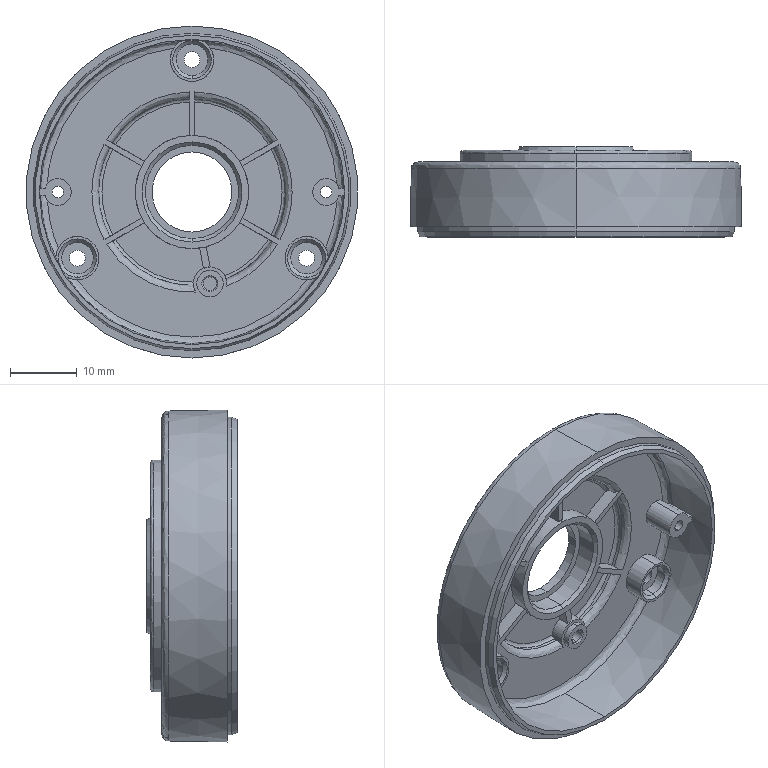Part | SolidWorks | features BaseBody 1 | 1 solid | 144 faces | box 49.792 x 13.5 x 49.792 mm | volume 7073 mm3 | cylinder 48 | plane 44 | cone 31 | spline 21 | commonest cylinder face diameters 4 x8 6.5 x7 2.4 x6 4.2 x6 4.75 x6 1.7 x4